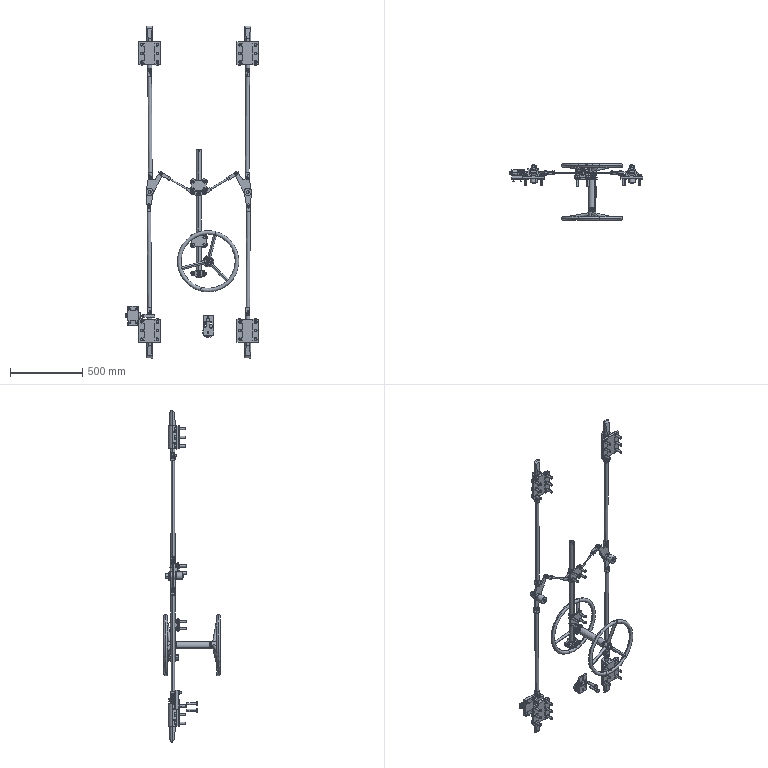Part | SolidWorks | features CompositeCurve 5 | 231 solids | 3632 faces | volume 8515021 mm3 | plane 1649 | cylinder 1140 | cone 701 | torus 140 | spline 2 | commonest cylinder face diameters 10 x124 18 x112 26 x100 14 x84 16 x80 44 x76